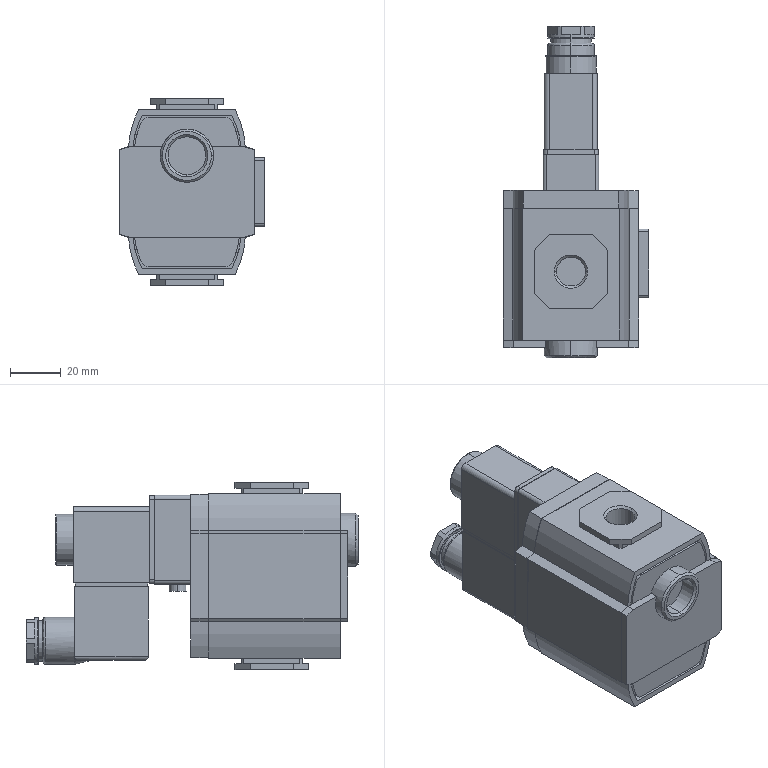Part | STEP file | soft-start valve GV30008JF1B | 2 solids | 206 faces | box 57.4 x 130.9 x 74 mm | volume 252989 mm3 | plane 132 | cylinder 59 | cone 9 | spline 6 | commonest cylinder face diameters 3 x13 2 x4 6 x4 11.445 x4 63.147 x4 65.1 x4